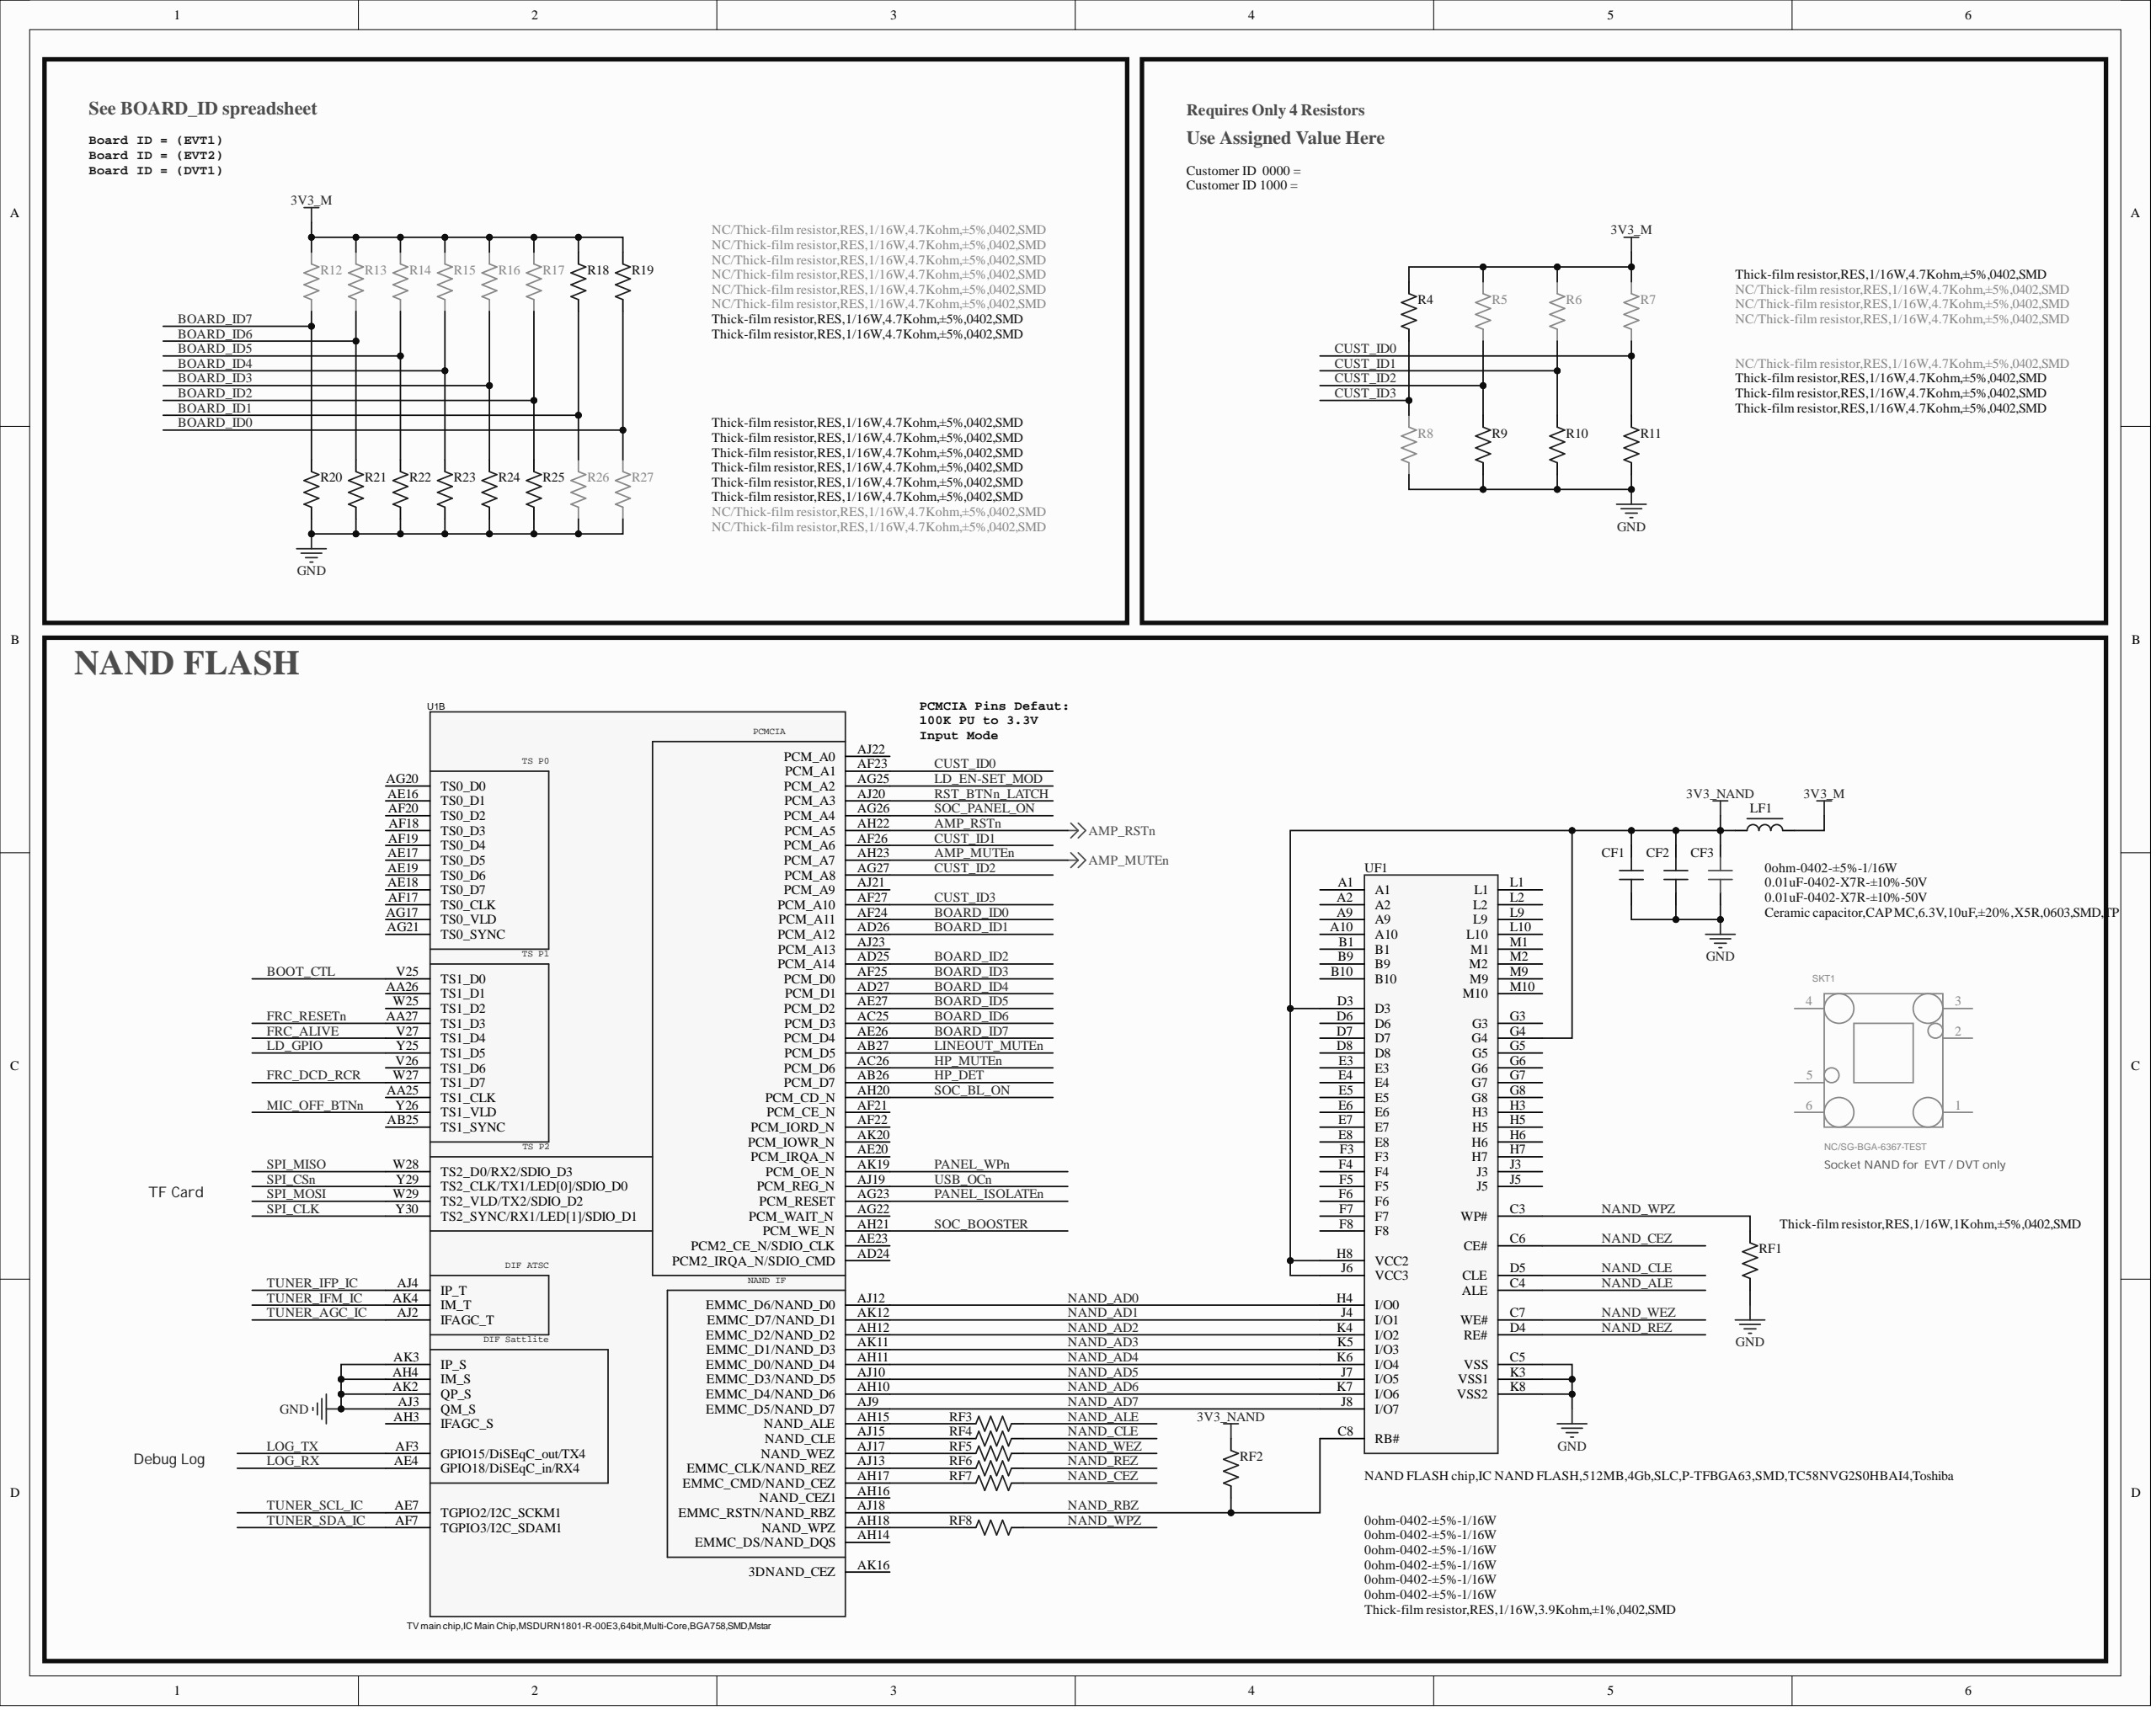Circuit board | Altium Designer | 1029 parts | 642 nets | one sheet of the schematic
Parts on this sheet (reference | value | footprint):
CF1 | 0.01uF-0402-X7R-±10%-50V | C0402
CF2 | 0.01uF-0402-X7R-±10%-50V | C0402
CF3 | Ceramic capacitor,CAP MC,6.3V,10uF,±20%,X5R,0603,SMD,TP | C0603
LF1 | 0ohm-0402-±5%-1/16W | L0402
R4 | Thick-film resistor,RES,1/16W,4.7Kohm,±5%,0402,SMD | R0402
R5 | NC/Thick-film resistor,RES,1/16W,4.7Kohm,±5%,0402,SMD | R0402
R6 | NC/Thick-film resistor,RES,1/16W,4.7Kohm,±5%,0402,SMD | R0402
R7 | NC/Thick-film resistor,RES,1/16W,4.7Kohm,±5%,0402,SMD | R0402
R8 | NC/Thick-film resistor,RES,1/16W,4.7Kohm,±5%,0402,SMD | R0402
R9 | Thick-film resistor,RES,1/16W,4.7Kohm,±5%,0402,SMD | R0402
R10 | Thick-film resistor,RES,1/16W,4.7Kohm,±5%,0402,SMD | R0402
R11 | Thick-film resistor,RES,1/16W,4.7Kohm,±5%,0402,SMD | R0402
R12 | NC/Thick-film resistor,RES,1/16W,4.7Kohm,±5%,0402,SMD | R0402
R13 | NC/Thick-film resistor,RES,1/16W,4.7Kohm,±5%,0402,SMD | R0402
R14 | NC/Thick-film resistor,RES,1/16W,4.7Kohm,±5%,0402,SMD | R0402
R15 | NC/Thick-film resistor,RES,1/16W,4.7Kohm,±5%,0402,SMD | R0402
R16 | NC/Thick-film resistor,RES,1/16W,4.7Kohm,±5%,0402,SMD | R0402
R17 | NC/Thick-film resistor,RES,1/16W,4.7Kohm,±5%,0402,SMD | R0402
R18 | Thick-film resistor,RES,1/16W,4.7Kohm,±5%,0402,SMD | R0402
R19 | Thick-film resistor,RES,1/16W,4.7Kohm,±5%,0402,SMD | R0402
R20 | Thick-film resistor,RES,1/16W,4.7Kohm,±5%,0402,SMD | R0402
R21 | Thick-film resistor,RES,1/16W,4.7Kohm,±5%,0402,SMD | R0402
R22 | Thick-film resistor,RES,1/16W,4.7Kohm,±5%,0402,SMD | R0402
R23 | Thick-film resistor,RES,1/16W,4.7Kohm,±5%,0402,SMD | R0402
R24 | Thick-film resistor,RES,1/16W,4.7Kohm,±5%,0402,SMD | R0402
R25 | Thick-film resistor,RES,1/16W,4.7Kohm,±5%,0402,SMD | R0402
R26 | NC/Thick-film resistor,RES,1/16W,4.7Kohm,±5%,0402,SMD | R0402
R27 | NC/Thick-film resistor,RES,1/16W,4.7Kohm,±5%,0402,SMD | R0402
RF1 | Thick-film resistor,RES,1/16W,1Kohm,±5%,0402,SMD | R0402
RF2 | Thick-film resistor,RES,1/16W,3.9Kohm,±1%,0402,SMD | R0402
RF3 | 0ohm-0402-±5%-1/16W | R0402
RF4 | 0ohm-0402-±5%-1/16W | R0402
RF5 | 0ohm-0402-±5%-1/16W | R0402
RF6 | 0ohm-0402-±5%-1/16W | R0402
RF7 | 0ohm-0402-±5%-1/16W | R0402
RF8 | 0ohm-0402-±5%-1/16W | R0402
SKT1 | NC/SG-BGA-6367-TEST | TEST-SG-BGA-6367
U1 | TV main chip,IC Main Chip,MSDURN1801-R-00E3,64bit,Multi-Core,BGA758,SMD,Mstar | BGA758/0.65
UF1 | NAND FLASH chip,IC NAND FLASH,512MB,4Gb,SLC,P-TFBGA63,SMD,TC58NVG2S0HBAI4,Toshiba | BGA63/0.8-1
Nets of these parts (net: part-pin ...):
USB_OCn: U1-AJ19
TUNER_SDA_IC: U1-AF7
TUNER_SCL_IC: U1-AE7
TUNER_IFP_IC: U1-AJ4
TUNER_IFM_IC: U1-AK4
TUNER_AGC_IC: U1-AJ2
SOC_PANEL_ON: U1-AG26
SOC_BOOSTER: U1-AH21
SOC_BL_ON: U1-AH20
RST_BTNn_LATCH: U1-AJ20
PANEL_ISOLATEn: U1-AG23
NetRF8_1: RF8-1 U1-AH18
NetRF7_1: RF7-1 U1-AH17
NetRF6_1: RF6-1 U1-AJ13
NetRF5_1: RF5-1 U1-AJ17
NetRF4_1: RF4-1 U1-AJ15
NetRF3_1: RF3-1 U1-AH15
NAND_WPZ: RF1-2 RF8-2 UF1-C3
NAND_WEZ: RF5-2 UF1-C7
NAND_REZ: RF6-2 UF1-D4
NAND_RBZ: RF2-1 U1-AJ18 UF1-C8
NAND_CLE: RF4-2 UF1-D5
NAND_CEZ: RF7-2 UF1-C6
NAND_ALE: RF3-2 UF1-C4
NAND_AD7: U1-AJ9 UF1-J8
NAND_AD6: U1-AH10 UF1-K7
NAND_AD5: U1-AJ10 UF1-J7
NAND_AD4: U1-AH11 UF1-K6
NAND_AD3: U1-AK11 UF1-K5
NAND_AD2: U1-AH12 UF1-K4
NAND_AD1: U1-AK12 UF1-J4
NAND_AD0: U1-AJ12 UF1-H4
LOG_TX: U1-AF3
LOG_RX: U1-AE4
LINEOUT_MUTEn: U1-AB27
LD_GPIO: U1-Y25
HP_MUTEn: U1-AC26
HP_DET: U1-AB26
GND: CF1-1 CF2-1 CF3-1 R8-1 R9-1 R10-1 R11-1 R20-1 R21-1 R22-1 R23-1 R24-1 R25-1 R26-1 R27-1 RF1-1 U1-AH4 U1-AJ3 U1-AK2 U1-AK3 U1-C3 U1-D6 U1-D8 U1-F6 U1-H6 U1-J4 U1-J5 U1-J6 U1-J7 U1-J8 U1-K7 U1-K8 U1-L9 U1-P1 U1-R4 U1-R8 U1-R9 U1-R10 U1-R18 U1-R19 U1-R20 U1-R21 U1-R22 U1-R23 U1-R24 U1-R25 U1-R26 U1-R27 UF1-C5 UF1-K3 UF1-K8
FRC_RESETn: U1-AA27
FRC_DCD_RCR: U1-W27
FRC_ALIVE: U1-V27
CUST_ID3: R4-1 R8-2 U1-AF27
CUST_ID2: R5-1 R9-2 U1-AG27
CUST_ID1: R6-1 R10-2 U1-AF26
CUST_ID0: R7-1 R11-2 U1-AF23
BOARD_ID7: R12-1 R20-2 U1-AE26
BOARD_ID6: R13-1 R21-2 U1-AC25
BOARD_ID5: R14-1 R22-2 U1-AE27
BOARD_ID4: R15-1 R23-2 U1-AD27
BOARD_ID3: R16-1 R24-2 U1-AF25
BOARD_ID2: R17-1 R25-2 U1-AD25
BOARD_ID1: R18-1 R26-2 U1-AD26
BOARD_ID0: R19-1 R27-2 U1-AF24
AMP_RSTn: U1-AH22
AMP_MUTEn: U1-AH23
3V3_NAND: CF1-2 CF2-2 CF3-2 LF1-1 RF2-2 UF1-D3 UF1-G4 UF1-H8 UF1-J6
3V3_M: LF1-2 R4-2 R5-2 R6-2 R7-2 R12-2 R13-2 R14-2 R15-2 R16-2 R17-2 R18-2 R19-2